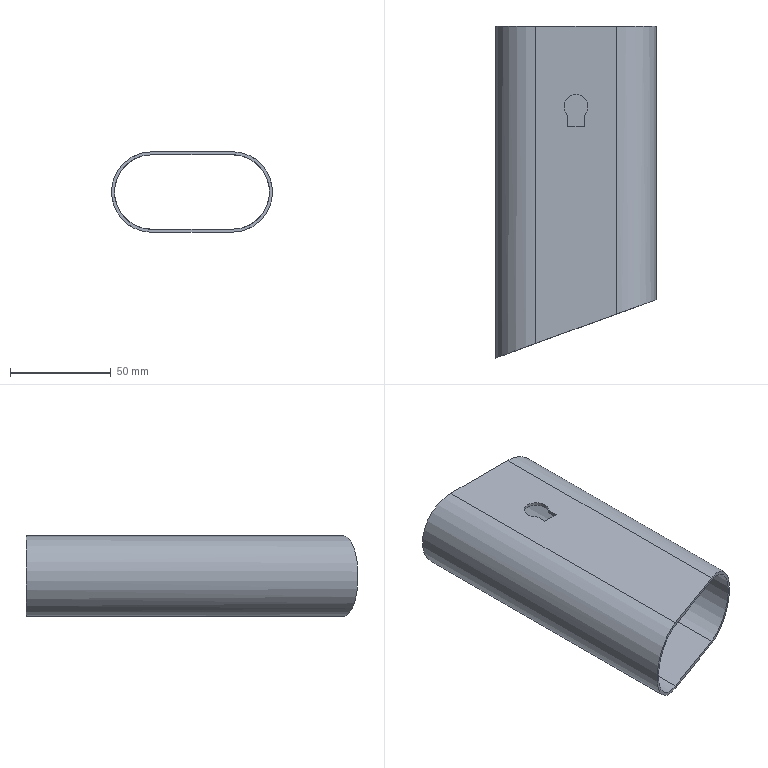Part | STEP file | 6100104R | 1 solid | 14 faces | box 80 x 165 x 40 mm | volume 45123 mm3 | plane 9 | cylinder 5 | commonest cylinder face diameters 37 x2 40 x2 12 x1
STEP:
#1=CARTESIAN_POINT('',(0.,0.,0.));
#2=DIRECTION('',(0.,0.,1.));
#3=DIRECTION('',(1.,0.,0.));
#4=AXIS2_PLACEMENT_3D('',#1,#2,#3);
#5=CARTESIAN_POINT('',(-20.,7.279,20.));
#6=VERTEX_POINT('',#5);
#7=CARTESIAN_POINT('',(-20.,7.279,-20.));
#8=VERTEX_POINT('',#7);
#9=CARTESIAN_POINT('',(-20.,7.279,20.));
#10=CARTESIAN_POINT('',(-60.,-7.279,20.));
#11=CARTESIAN_POINT('',(-60.,-7.279,-20.));
#12=CARTESIAN_POINT('',(-20.,7.279,-20.));
#13=(BOUNDED_CURVE()B_SPLINE_CURVE(3,(#9,#10,#11,#12),.UNSPECIFIED.,.F.,.F.)B_SPLINE_CURVE_WITH_KNOTS((4,4),(4.712,7.854),.PIECEWISE_BEZIER_KNOTS.)CURVE()GEOMETRIC_REPRESENTATION_ITEM()RATIONAL_B_SPLINE_CURVE((1.,0.3333,0.3333,1.))REPRESENTATION_ITEM(''));
#14=CARTESIAN_POINT('',(-20.,165.,0.));
#15=DIRECTION('',(0.,-1.,0.));
#16=DIRECTION('',(0.,0.,-1.));
#17=AXIS2_PLACEMENT_3D('',#14,#15,#16);
#18=CYLINDRICAL_SURFACE('',#17,20.);
#19=CARTESIAN_POINT('',(3.142,157.721));
#20=CARTESIAN_POINT('',(3.172,157.941));
#21=CARTESIAN_POINT('',(3.235,158.403));
#22=CARTESIAN_POINT('',(3.339,159.153));
#23=CARTESIAN_POINT('',(3.453,159.957));
#24=CARTESIAN_POINT('',(3.577,160.8));
#25=CARTESIAN_POINT('',(3.712,161.664));
#26=CARTESIAN_POINT('',(3.857,162.516));
#27=CARTESIAN_POINT('',(4.013,163.316));
#28=CARTESIAN_POINT('',(4.179,164.017));
#29=CARTESIAN_POINT('',(4.352,164.567));
#30=CARTESIAN_POINT('',(4.531,164.919));
#31=CARTESIAN_POINT('',(4.712,165.04));
#32=CARTESIAN_POINT('',(4.894,164.919));
#33=CARTESIAN_POINT('',(5.073,164.567));
#34=CARTESIAN_POINT('',(5.246,164.017));
#35=CARTESIAN_POINT('',(5.412,163.316));
#36=CARTESIAN_POINT('',(5.567,162.516));
#37=CARTESIAN_POINT('',(5.713,161.664));
#38=CARTESIAN_POINT('',(5.848,160.8));
#39=CARTESIAN_POINT('',(5.972,159.957));
#40=CARTESIAN_POINT('',(6.085,159.153));
#41=CARTESIAN_POINT('',(6.19,158.403));
#42=CARTESIAN_POINT('',(6.253,157.941));
#43=CARTESIAN_POINT('',(6.283,157.721));
#44=B_SPLINE_CURVE_WITH_KNOTS('',3,(#19,#20,#21,#22,#23,#24,#25,#26,#27,#28,#29,#30,#31,#32,#33,#34,#35,#36,#37,#38,#39,#40,#41,#42,#43),.UNSPECIFIED.,.F.,.F.,(4,1,1,1,1,1,1,1,1,1,1,1,1,1,1,1,1,1,1,1,1,1,4),(4.712,4.855,4.998,5.141,5.284,5.426,5.569,5.712,5.855,5.998,6.14,6.283,6.426,6.569,6.712,6.854,6.997,7.14,7.283,7.426,7.568,7.711,7.854),.QUASI_UNIFORM_KNOTS.);
#45=(GEOMETRIC_REPRESENTATION_CONTEXT(2)PARAMETRIC_REPRESENTATION_CONTEXT()REPRESENTATION_CONTEXT('',''));
#46=DEFINITIONAL_REPRESENTATION('',(#44),#45);
#47=PCURVE('',#18,#46);
#48=CARTESIAN_POINT('',(-40.,0.,-40.));
#49=DIRECTION('',(0.342,-0.9397,0.));
#50=DIRECTION('',(0.9397,0.342,0.));
#51=AXIS2_PLACEMENT_3D('',#48,#49,#50);
#52=PLANE('',#51);
#53=CARTESIAN_POINT('',(21.284,60.));
#54=CARTESIAN_POINT('',(-21.284,60.));
#55=CARTESIAN_POINT('',(-21.284,20.));
#56=CARTESIAN_POINT('',(21.284,20.));
#57=(BOUNDED_CURVE()B_SPLINE_CURVE(3,(#53,#54,#55,#56),.UNSPECIFIED.,.F.,.F.)B_SPLINE_CURVE_WITH_KNOTS((4,4),(4.712,7.854),.PIECEWISE_BEZIER_KNOTS.)CURVE()GEOMETRIC_REPRESENTATION_ITEM()RATIONAL_B_SPLINE_CURVE((1.,0.3333,0.3333,1.))REPRESENTATION_ITEM(''));
#58=(GEOMETRIC_REPRESENTATION_CONTEXT(2)PARAMETRIC_REPRESENTATION_CONTEXT()REPRESENTATION_CONTEXT('',''));
#59=DEFINITIONAL_REPRESENTATION('',(#57),#58);
#60=PCURVE('',#52,#59);
#61=SURFACE_CURVE('',#13,(#47,#60),.PCURVE_S1.);
#62=EDGE_CURVE('',#6,#8,#61,.T.);
#63=ORIENTED_EDGE('',*,*,#62,.F.);
#64=CARTESIAN_POINT('',(-20.,165.,20.));
#65=VERTEX_POINT('',#64);
#66=CARTESIAN_POINT('',(-20.,165.,20.));
#67=DIRECTION('',(0.,-1.,0.));
#68=VECTOR('',#67,1.);
#69=LINE('',#66,#68);
#70=CARTESIAN_POINT('',(3.142,0.));
#71=DIRECTION('',(0.,1.));
#72=VECTOR('',#71,1.);
#73=LINE('',#70,#72);
#74=(GEOMETRIC_REPRESENTATION_CONTEXT(2)PARAMETRIC_REPRESENTATION_CONTEXT()REPRESENTATION_CONTEXT('',''));
#75=DEFINITIONAL_REPRESENTATION('',(#73),#74);
#76=PCURVE('',#18,#75);
#77=CARTESIAN_POINT('',(-20.,165.,20.));
#78=DIRECTION('',(0.,0.,-1.));
#79=DIRECTION('',(-1.,0.,0.));
#80=AXIS2_PLACEMENT_3D('',#77,#78,#79);
#81=PLANE('',#80);
#82=CARTESIAN_POINT('',(0.,0.));
#83=DIRECTION('',(0.,-1.));
#84=VECTOR('',#83,1.);
#85=LINE('',#82,#84);
#86=(GEOMETRIC_REPRESENTATION_CONTEXT(2)PARAMETRIC_REPRESENTATION_CONTEXT()REPRESENTATION_CONTEXT('',''));
#87=DEFINITIONAL_REPRESENTATION('',(#85),#86);
#88=PCURVE('',#81,#87);
#89=SURFACE_CURVE('',#69,(#76,#88),.PCURVE_S1.);
#90=EDGE_CURVE('',#65,#6,#89,.T.);
#91=ORIENTED_EDGE('',*,*,#90,.F.);
#92=CARTESIAN_POINT('',(-20.,165.,-20.));
#93=VERTEX_POINT('',#92);
#94=CARTESIAN_POINT('',(-20.,165.,0.));
#95=DIRECTION('',(0.,1.,0.));
#96=DIRECTION('',(0.,0.,1.));
#97=AXIS2_PLACEMENT_3D('',#94,#95,#96);
#98=CIRCLE('',#97,20.);
#99=CARTESIAN_POINT('',(9.425,0.));
#100=DIRECTION('',(-1.,0.));
#101=VECTOR('',#100,1.);
#102=LINE('',#99,#101);
#103=(GEOMETRIC_REPRESENTATION_CONTEXT(2)PARAMETRIC_REPRESENTATION_CONTEXT()REPRESENTATION_CONTEXT('',''));
#104=DEFINITIONAL_REPRESENTATION('',(#102),#103);
#105=PCURVE('',#18,#104);
#106=CARTESIAN_POINT('',(-20.,165.,0.));
#107=DIRECTION('',(0.,1.,0.));
#108=DIRECTION('',(0.,0.,1.));
#109=AXIS2_PLACEMENT_3D('',#106,#107,#108);
#110=PLANE('',#109);
#111=CARTESIAN_POINT('',(0.,0.));
#112=DIRECTION('',(1.,0.));
#113=AXIS2_PLACEMENT_2D('',#111,#112);
#114=CIRCLE('',#113,20.);
#115=(GEOMETRIC_REPRESENTATION_CONTEXT(2)PARAMETRIC_REPRESENTATION_CONTEXT()REPRESENTATION_CONTEXT('',''));
#116=DEFINITIONAL_REPRESENTATION('',(#114),#115);
#117=PCURVE('',#110,#116);
#118=SURFACE_CURVE('',#98,(#105,#117),.PCURVE_S1.);
#119=EDGE_CURVE('',#93,#65,#118,.T.);
#120=ORIENTED_EDGE('',*,*,#119,.F.);
#121=CARTESIAN_POINT('',(-20.,165.,-20.));
#122=DIRECTION('',(0.,-1.,0.));
#123=VECTOR('',#122,1.);
#124=LINE('',#121,#123);
#125=CARTESIAN_POINT('',(6.283,0.));
#126=DIRECTION('',(0.,1.));
#127=VECTOR('',#126,1.);
#128=LINE('',#125,#127);
#129=(GEOMETRIC_REPRESENTATION_CONTEXT(2)PARAMETRIC_REPRESENTATION_CONTEXT()REPRESENTATION_CONTEXT('',''));
#130=DEFINITIONAL_REPRESENTATION('',(#128),#129);
#131=PCURVE('',#18,#130);
#132=CARTESIAN_POINT('',(-20.,165.,-20.));
#133=DIRECTION('',(0.,0.,1.));
#134=DIRECTION('',(1.,0.,0.));
#135=AXIS2_PLACEMENT_3D('',#132,#133,#134);
#136=PLANE('',#135);
#137=CARTESIAN_POINT('',(0.,0.));
#138=DIRECTION('',(0.,-1.));
#139=VECTOR('',#138,1.);
#140=LINE('',#137,#139);
#141=(GEOMETRIC_REPRESENTATION_CONTEXT(2)PARAMETRIC_REPRESENTATION_CONTEXT()REPRESENTATION_CONTEXT('',''));
#142=DEFINITIONAL_REPRESENTATION('',(#140),#141);
#143=PCURVE('',#136,#142);
#144=SURFACE_CURVE('',#124,(#131,#143),.PCURVE_S1.);
#145=EDGE_CURVE('',#93,#8,#144,.T.);
#146=ORIENTED_EDGE('',*,*,#145,.T.);
#147=EDGE_LOOP('',(#63,#91,#120,#146));
#148=FACE_BOUND('',#147,.T.);
#149=ADVANCED_FACE('',(#148),#18,.T.);
#150=CARTESIAN_POINT('',(4.,120.528,20.));
#151=VERTEX_POINT('',#150);
#152=CARTESIAN_POINT('',(-4.,120.528,20.));
#153=VERTEX_POINT('',#152);
#154=CARTESIAN_POINT('',(0.,125.,20.));
#155=DIRECTION('',(0.,0.,1.));
#156=DIRECTION('',(-1.,0.,0.));
#157=AXIS2_PLACEMENT_3D('',#154,#155,#156);
#158=CIRCLE('',#157,6.);
#159=CARTESIAN_POINT('',(-14.,-40.));
#160=CARTESIAN_POINT('',(-14.,-50.392));
#161=CARTESIAN_POINT('',(-23.,-45.196));
#162=CARTESIAN_POINT('',(-32.,-40.));
#163=CARTESIAN_POINT('',(-23.,-34.804));
#164=CARTESIAN_POINT('',(-14.,-29.608));
#165=CARTESIAN_POINT('',(-14.,-40.));
#166=(BOUNDED_CURVE()B_SPLINE_CURVE(2,(#159,#160,#161,#162,#163,#164,#165),.UNSPECIFIED.,.T.,.F.)B_SPLINE_CURVE_WITH_KNOTS((1,2,2,2,2,1),(-2.094,0.,2.094,4.189,6.283,8.378),.UNSPECIFIED.)CURVE()GEOMETRIC_REPRESENTATION_ITEM()RATIONAL_B_SPLINE_CURVE((1.,0.5,1.,0.5,1.,0.5,1.))REPRESENTATION_ITEM(''));
#167=(GEOMETRIC_REPRESENTATION_CONTEXT(2)PARAMETRIC_REPRESENTATION_CONTEXT()REPRESENTATION_CONTEXT('',''));
#168=DEFINITIONAL_REPRESENTATION('',(#166),#167);
#169=PCURVE('',#81,#168);
#170=CARTESIAN_POINT('',(0.,125.,40.));
#171=DIRECTION('',(0.,0.,-1.));
#172=DIRECTION('',(-1.,0.,0.));
#173=AXIS2_PLACEMENT_3D('',#170,#171,#172);
#174=CYLINDRICAL_SURFACE('',#173,6.);
#175=CARTESIAN_POINT('',(6.283,20.));
#176=DIRECTION('',(-1.,0.));
#177=VECTOR('',#176,1.);
#178=LINE('',#175,#177);
#179=(GEOMETRIC_REPRESENTATION_CONTEXT(2)PARAMETRIC_REPRESENTATION_CONTEXT()REPRESENTATION_CONTEXT('',''));
#180=DEFINITIONAL_REPRESENTATION('',(#178),#179);
#181=PCURVE('',#174,#180);
#182=SURFACE_CURVE('',#158,(#169,#181),.PCURVE_S1.);
#183=EDGE_CURVE('',#151,#153,#182,.T.);
#184=ORIENTED_EDGE('',*,*,#183,.F.);
#185=CARTESIAN_POINT('',(4.,115.,20.));
#186=VERTEX_POINT('',#185);
#187=CARTESIAN_POINT('',(4.,165.,20.));
#188=DIRECTION('',(0.,-1.,0.));
#189=VECTOR('',#188,1.);
#190=LINE('',#187,#189);
#191=CARTESIAN_POINT('',(-24.,0.));
#192=DIRECTION('',(0.,-1.));
#193=VECTOR('',#192,1.);
#194=LINE('',#191,#193);
#195=(GEOMETRIC_REPRESENTATION_CONTEXT(2)PARAMETRIC_REPRESENTATION_CONTEXT()REPRESENTATION_CONTEXT('',''));
#196=DEFINITIONAL_REPRESENTATION('',(#194),#195);
#197=PCURVE('',#81,#196);
#198=CARTESIAN_POINT('',(4.,120.528,40.));
#199=DIRECTION('',(1.,0.,0.));
#200=DIRECTION('',(0.,1.,0.));
#201=AXIS2_PLACEMENT_3D('',#198,#199,#200);
#202=PLANE('',#201);
#203=CARTESIAN_POINT('',(44.472,-20.));
#204=DIRECTION('',(-1.,0.));
#205=VECTOR('',#204,1.);
#206=LINE('',#203,#205);
#207=(GEOMETRIC_REPRESENTATION_CONTEXT(2)PARAMETRIC_REPRESENTATION_CONTEXT()REPRESENTATION_CONTEXT('',''));
#208=DEFINITIONAL_REPRESENTATION('',(#206),#207);
#209=PCURVE('',#202,#208);
#210=SURFACE_CURVE('',#190,(#197,#209),.PCURVE_S1.);
#211=EDGE_CURVE('',#151,#186,#210,.T.);
#212=ORIENTED_EDGE('',*,*,#211,.T.);
#213=CARTESIAN_POINT('',(-4.,115.,20.));
#214=VERTEX_POINT('',#213);
#215=CARTESIAN_POINT('',(-20.,115.,20.));
#216=DIRECTION('',(1.,0.,0.));
#217=VECTOR('',#216,1.);
#218=LINE('',#215,#217);
#219=CARTESIAN_POINT('',(0.,-50.));
#220=DIRECTION('',(-1.,0.));
#221=VECTOR('',#220,1.);
#222=LINE('',#219,#221);
#223=(GEOMETRIC_REPRESENTATION_CONTEXT(2)PARAMETRIC_REPRESENTATION_CONTEXT()REPRESENTATION_CONTEXT('',''));
#224=DEFINITIONAL_REPRESENTATION('',(#222),#223);
#225=PCURVE('',#81,#224);
#226=CARTESIAN_POINT('',(-4.,115.,40.));
#227=DIRECTION('',(0.,1.,0.));
#228=DIRECTION('',(0.,0.,1.));
#229=AXIS2_PLACEMENT_3D('',#226,#227,#228);
#230=PLANE('',#229);
#231=CARTESIAN_POINT('',(-20.,-16.));
#232=DIRECTION('',(0.,1.));
#233=VECTOR('',#232,1.);
#234=LINE('',#231,#233);
#235=(GEOMETRIC_REPRESENTATION_CONTEXT(2)PARAMETRIC_REPRESENTATION_CONTEXT()REPRESENTATION_CONTEXT('',''));
#236=DEFINITIONAL_REPRESENTATION('',(#234),#235);
#237=PCURVE('',#230,#236);
#238=SURFACE_CURVE('',#218,(#225,#237),.PCURVE_S1.);
#239=EDGE_CURVE('',#214,#186,#238,.T.);
#240=ORIENTED_EDGE('',*,*,#239,.F.);
#241=CARTESIAN_POINT('',(-4.,165.,20.));
#242=DIRECTION('',(0.,-1.,0.));
#243=VECTOR('',#242,1.);
#244=LINE('',#241,#243);
#245=CARTESIAN_POINT('',(-16.,0.));
#246=DIRECTION('',(0.,-1.));
#247=VECTOR('',#246,1.);
#248=LINE('',#245,#247);
#249=(GEOMETRIC_REPRESENTATION_CONTEXT(2)PARAMETRIC_REPRESENTATION_CONTEXT()REPRESENTATION_CONTEXT('',''));
#250=DEFINITIONAL_REPRESENTATION('',(#248),#249);
#251=PCURVE('',#81,#250);
#252=CARTESIAN_POINT('',(-4.,120.528,40.));
#253=DIRECTION('',(1.,0.,0.));
#254=DIRECTION('',(0.,1.,0.));
#255=AXIS2_PLACEMENT_3D('',#252,#253,#254);
#256=PLANE('',#255);
#257=CARTESIAN_POINT('',(44.472,-20.));
#258=DIRECTION('',(-1.,0.));
#259=VECTOR('',#258,1.);
#260=LINE('',#257,#259);
#261=(GEOMETRIC_REPRESENTATION_CONTEXT(2)PARAMETRIC_REPRESENTATION_CONTEXT()REPRESENTATION_CONTEXT('',''));
#262=DEFINITIONAL_REPRESENTATION('',(#260),#261);
#263=PCURVE('',#256,#262);
#264=SURFACE_CURVE('',#244,(#251,#263),.PCURVE_S1.);
#265=EDGE_CURVE('',#153,#214,#264,.T.);
#266=ORIENTED_EDGE('',*,*,#265,.F.);
#267=EDGE_LOOP('',(#184,#212,#240,#266));
#268=FACE_BOUND('',#267,.T.);
#269=CARTESIAN_POINT('',(20.,21.838,20.));
#270=VERTEX_POINT('',#269);
#271=CARTESIAN_POINT('',(30.69,25.729,20.));
#272=DIRECTION('',(-0.9397,-0.342,0.));
#273=VECTOR('',#272,1.);
#274=LINE('',#271,#273);
#275=CARTESIAN_POINT('',(-50.69,-139.271));
#276=DIRECTION('',(0.9397,-0.342));
#277=VECTOR('',#276,1.);
#278=LINE('',#275,#277);
#279=(GEOMETRIC_REPRESENTATION_CONTEXT(2)PARAMETRIC_REPRESENTATION_CONTEXT()REPRESENTATION_CONTEXT('',''));
#280=DEFINITIONAL_REPRESENTATION('',(#278),#279);
#281=PCURVE('',#81,#280);
#282=CARTESIAN_POINT('',(75.227,60.));
#283=DIRECTION('',(-1.,0.));
#284=VECTOR('',#283,1.);
#285=LINE('',#282,#284);
#286=(GEOMETRIC_REPRESENTATION_CONTEXT(2)PARAMETRIC_REPRESENTATION_CONTEXT()REPRESENTATION_CONTEXT('',''));
#287=DEFINITIONAL_REPRESENTATION('',(#285),#286);
#288=PCURVE('',#52,#287);
#289=SURFACE_CURVE('',#274,(#281,#288),.PCURVE_S1.);
#290=EDGE_CURVE('',#270,#6,#289,.T.);
#291=ORIENTED_EDGE('',*,*,#290,.F.);
#292=CARTESIAN_POINT('',(20.,165.,20.));
#293=VERTEX_POINT('',#292);
#294=CARTESIAN_POINT('',(20.,165.,20.));
#295=DIRECTION('',(0.,-1.,0.));
#296=VECTOR('',#295,1.);
#297=LINE('',#294,#296);
#298=CARTESIAN_POINT('',(-40.,0.));
#299=DIRECTION('',(0.,-1.));
#300=VECTOR('',#299,1.);
#301=LINE('',#298,#300);
#302=(GEOMETRIC_REPRESENTATION_CONTEXT(2)PARAMETRIC_REPRESENTATION_CONTEXT()REPRESENTATION_CONTEXT('',''));
#303=DEFINITIONAL_REPRESENTATION('',(#301),#302);
#304=PCURVE('',#81,#303);
#305=CARTESIAN_POINT('',(20.,165.,0.));
#306=DIRECTION('',(0.,-1.,0.));
#307=DIRECTION('',(0.,0.,-1.));
#308=AXIS2_PLACEMENT_3D('',#305,#306,#307);
#309=CYLINDRICAL_SURFACE('',#308,20.);
#310=CARTESIAN_POINT('',(3.142,0.));
#311=DIRECTION('',(0.,1.));
#312=VECTOR('',#311,1.);
#313=LINE('',#310,#312);
#314=(GEOMETRIC_REPRESENTATION_CONTEXT(2)PARAMETRIC_REPRESENTATION_CONTEXT()REPRESENTATION_CONTEXT('',''));
#315=DEFINITIONAL_REPRESENTATION('',(#313),#314);
#316=PCURVE('',#309,#315);
#317=SURFACE_CURVE('',#297,(#304,#316),.PCURVE_S1.);
#318=EDGE_CURVE('',#293,#270,#317,.T.);
#319=ORIENTED_EDGE('',*,*,#318,.F.);
#320=CARTESIAN_POINT('',(-20.,165.,20.));
#321=DIRECTION('',(1.,0.,0.));
#322=VECTOR('',#321,1.);
#323=LINE('',#320,#322);
#324=CARTESIAN_POINT('',(0.,0.));
#325=DIRECTION('',(-1.,0.));
#326=VECTOR('',#325,1.);
#327=LINE('',#324,#326);
#328=(GEOMETRIC_REPRESENTATION_CONTEXT(2)PARAMETRIC_REPRESENTATION_CONTEXT()REPRESENTATION_CONTEXT('',''));
#329=DEFINITIONAL_REPRESENTATION('',(#327),#328);
#330=PCURVE('',#81,#329);
#331=CARTESIAN_POINT('',(20.,0.));
#332=DIRECTION('',(0.,1.));
#333=VECTOR('',#332,1.);
#334=LINE('',#331,#333);
#335=(GEOMETRIC_REPRESENTATION_CONTEXT(2)PARAMETRIC_REPRESENTATION_CONTEXT()REPRESENTATION_CONTEXT('',''));
#336=DEFINITIONAL_REPRESENTATION('',(#334),#335);
#337=PCURVE('',#110,#336);
#338=SURFACE_CURVE('',#323,(#330,#337),.PCURVE_S1.);
#339=EDGE_CURVE('',#65,#293,#338,.T.);
#340=ORIENTED_EDGE('',*,*,#339,.F.);
#341=ORIENTED_EDGE('',*,*,#90,.T.);
#342=EDGE_LOOP('',(#291,#319,#340,#341));
#343=FACE_BOUND('',#342,.T.);
#344=ADVANCED_FACE('',(#268,#343),#81,.F.);
#345=ORIENTED_EDGE('',*,*,#318,.T.);
#346=CARTESIAN_POINT('',(20.,21.838,-20.));
#347=VERTEX_POINT('',#346);
#348=CARTESIAN_POINT('',(20.,21.838,-20.));
#349=CARTESIAN_POINT('',(60.,36.397,-20.));
#350=CARTESIAN_POINT('',(60.,36.397,20.));
#351=CARTESIAN_POINT('',(20.,21.838,20.));
#352=(BOUNDED_CURVE()B_SPLINE_CURVE(3,(#348,#349,#350,#351),.UNSPECIFIED.,.F.,.F.)B_SPLINE_CURVE_WITH_KNOTS((4,4),(1.571,4.712),.PIECEWISE_BEZIER_KNOTS.)CURVE()GEOMETRIC_REPRESENTATION_ITEM()RATIONAL_B_SPLINE_CURVE((1.,0.3333,0.3333,1.))REPRESENTATION_ITEM(''));
#353=CARTESIAN_POINT('',(0.,143.162));
#354=CARTESIAN_POINT('',(0.0303,142.942));
#355=CARTESIAN_POINT('',(0.09367,142.48));
#356=CARTESIAN_POINT('',(0.1977,141.729));
#357=CARTESIAN_POINT('',(0.3115,140.926));
#358=CARTESIAN_POINT('',(0.4356,140.082));
#359=CARTESIAN_POINT('',(0.5703,139.219));
#360=CARTESIAN_POINT('',(0.7158,138.367));
#361=CARTESIAN_POINT('',(0.8717,137.566));
#362=CARTESIAN_POINT('',(1.037,136.865));
#363=CARTESIAN_POINT('',(1.21,136.315));
#364=CARTESIAN_POINT('',(1.389,135.963));
#365=CARTESIAN_POINT('',(1.571,135.842));
#366=CARTESIAN_POINT('',(1.753,135.963));
#367=CARTESIAN_POINT('',(1.931,136.315));
#368=CARTESIAN_POINT('',(2.105,136.865));
#369=CARTESIAN_POINT('',(2.27,137.566));
#370=CARTESIAN_POINT('',(2.426,138.367));
#371=CARTESIAN_POINT('',(2.571,139.219));
#372=CARTESIAN_POINT('',(2.706,140.082));
#373=CARTESIAN_POINT('',(2.83,140.926));
#374=CARTESIAN_POINT('',(2.944,141.729));
#375=CARTESIAN_POINT('',(3.048,142.48));
#376=CARTESIAN_POINT('',(3.111,142.942));
#377=CARTESIAN_POINT('',(3.142,143.162));
#378=B_SPLINE_CURVE_WITH_KNOTS('',3,(#353,#354,#355,#356,#357,#358,#359,#360,#361,#362,#363,#364,#365,#366,#367,#368,#369,#370,#371,#372,#373,#374,#375,#376,#377),.UNSPECIFIED.,.F.,.F.,(4,1,1,1,1,1,1,1,1,1,1,1,1,1,1,1,1,1,1,1,1,1,4),(1.571,1.714,1.856,1.999,2.142,2.285,2.428,2.57,2.713,2.856,2.999,3.142,3.284,3.427,3.57,3.713,3.856,3.998,4.141,4.284,4.427,4.57,4.712),.QUASI_UNIFORM_KNOTS.);
#379=(GEOMETRIC_REPRESENTATION_CONTEXT(2)PARAMETRIC_REPRESENTATION_CONTEXT()REPRESENTATION_CONTEXT('',''));
#380=DEFINITIONAL_REPRESENTATION('',(#378),#379);
#381=PCURVE('',#309,#380);
#382=CARTESIAN_POINT('',(63.851,20.));
#383=CARTESIAN_POINT('',(106.418,20.));
#384=CARTESIAN_POINT('',(106.418,60.));
#385=CARTESIAN_POINT('',(63.851,60.));
#386=(BOUNDED_CURVE()B_SPLINE_CURVE(3,(#382,#383,#384,#385),.UNSPECIFIED.,.F.,.F.)B_SPLINE_CURVE_WITH_KNOTS((4,4),(1.571,4.712),.PIECEWISE_BEZIER_KNOTS.)CURVE()GEOMETRIC_REPRESENTATION_ITEM()RATIONAL_B_SPLINE_CURVE((1.,0.3333,0.3333,1.))REPRESENTATION_ITEM(''));
#387=(GEOMETRIC_REPRESENTATION_CONTEXT(2)PARAMETRIC_REPRESENTATION_CONTEXT()REPRESENTATION_CONTEXT('',''));
#388=DEFINITIONAL_REPRESENTATION('',(#386),#387);
#389=PCURVE('',#52,#388);
#390=SURFACE_CURVE('',#352,(#381,#389),.PCURVE_S1.);
#391=EDGE_CURVE('',#347,#270,#390,.T.);
#392=ORIENTED_EDGE('',*,*,#391,.F.);
#393=CARTESIAN_POINT('',(20.,165.,-20.));
#394=VERTEX_POINT('',#393);
#395=CARTESIAN_POINT('',(20.,165.,-20.));
#396=DIRECTION('',(0.,-1.,0.));
#397=VECTOR('',#396,1.);
#398=LINE('',#395,#397);
#399=CARTESIAN_POINT('',(0.,0.));
#400=DIRECTION('',(0.,1.));
#401=VECTOR('',#400,1.);
#402=LINE('',#399,#401);
#403=(GEOMETRIC_REPRESENTATION_CONTEXT(2)PARAMETRIC_REPRESENTATION_CONTEXT()REPRESENTATION_CONTEXT('',''));
#404=DEFINITIONAL_REPRESENTATION('',(#402),#403);
#405=PCURVE('',#309,#404);
#406=CARTESIAN_POINT('',(40.,0.));
#407=DIRECTION('',(0.,-1.));
#408=VECTOR('',#407,1.);
#409=LINE('',#406,#408);
#410=(GEOMETRIC_REPRESENTATION_CONTEXT(2)PARAMETRIC_REPRESENTATION_CONTEXT()REPRESENTATION_CONTEXT('',''));
#411=DEFINITIONAL_REPRESENTATION('',(#409),#410);
#412=PCURVE('',#136,#411);
#413=SURFACE_CURVE('',#398,(#405,#412),.PCURVE_S1.);
#414=EDGE_CURVE('',#394,#347,#413,.T.);
#415=ORIENTED_EDGE('',*,*,#414,.F.);
#416=CARTESIAN_POINT('',(20.,165.,0.));
#417=DIRECTION('',(0.,1.,0.));
#418=DIRECTION('',(0.,0.,1.));
#419=AXIS2_PLACEMENT_3D('',#416,#417,#418);
#420=CIRCLE('',#419,20.);
#421=CARTESIAN_POINT('',(3.142,0.));
#422=DIRECTION('',(-1.,0.));
#423=VECTOR('',#422,1.);
#424=LINE('',#421,#423);
#425=(GEOMETRIC_REPRESENTATION_CONTEXT(2)PARAMETRIC_REPRESENTATION_CONTEXT()REPRESENTATION_CONTEXT('',''));
#426=DEFINITIONAL_REPRESENTATION('',(#424),#425);
#427=PCURVE('',#309,#426);
#428=CARTESIAN_POINT('',(0.,40.));
#429=DIRECTION('',(1.,0.));
#430=AXIS2_PLACEMENT_2D('',#428,#429);
#431=CIRCLE('',#430,20.);
#432=(GEOMETRIC_REPRESENTATION_CONTEXT(2)PARAMETRIC_REPRESENTATION_CONTEXT()REPRESENTATION_CONTEXT('',''));
#433=DEFINITIONAL_REPRESENTATION('',(#431),#432);
#434=PCURVE('',#110,#433);
#435=SURFACE_CURVE('',#420,(#427,#434),.PCURVE_S1.);
#436=EDGE_CURVE('',#293,#394,#435,.T.);
#437=ORIENTED_EDGE('',*,*,#436,.F.);
#438=EDGE_LOOP('',(#345,#392,#415,#437));
#439=FACE_BOUND('',#438,.T.);
#440=ADVANCED_FACE('',(#439),#309,.T.);
#441=CARTESIAN_POINT('',(30.69,25.729,-20.));
#442=DIRECTION('',(0.9397,0.342,0.));
#443=VECTOR('',#442,1.);
#444=LINE('',#441,#443);
#445=CARTESIAN_POINT('',(50.69,-139.271));
#446=DIRECTION('',(0.9397,0.342));
#447=VECTOR('',#446,1.);
#448=LINE('',#445,#447);
#449=(GEOMETRIC_REPRESENTATION_CONTEXT(2)PARAMETRIC_REPRESENTATION_CONTEXT()REPRESENTATION_CONTEXT('',''));
#450=DEFINITIONAL_REPRESENTATION('',(#448),#449);
#451=PCURVE('',#136,#450);
#452=CARTESIAN_POINT('',(75.227,20.));
#453=DIRECTION('',(1.,0.));
#454=VECTOR('',#453,1.);
#455=LINE('',#452,#454);
#456=(GEOMETRIC_REPRESENTATION_CONTEXT(2)PARAMETRIC_REPRESENTATION_CONTEXT()REPRESENTATION_CONTEXT('',''));
#457=DEFINITIONAL_REPRESENTATION('',(#455),#456);
#458=PCURVE('',#52,#457);
#459=SURFACE_CURVE('',#444,(#451,#458),.PCURVE_S1.);
#460=EDGE_CURVE('',#8,#347,#459,.T.);
#461=ORIENTED_EDGE('',*,*,#460,.F.);
#462=ORIENTED_EDGE('',*,*,#145,.F.);
#463=CARTESIAN_POINT('',(-20.,165.,-20.));
#464=DIRECTION('',(-1.,0.,0.));
#465=VECTOR('',#464,1.);
#466=LINE('',#463,#465);
#467=CARTESIAN_POINT('',(0.,0.));
#468=DIRECTION('',(-1.,0.));
#469=VECTOR('',#468,1.);
#470=LINE('',#467,#469);
#471=(GEOMETRIC_REPRESENTATION_CONTEXT(2)PARAMETRIC_REPRESENTATION_CONTEXT()REPRESENTATION_CONTEXT('',''));
#472=DEFINITIONAL_REPRESENTATION('',(#470),#471);
#473=PCURVE('',#136,#472);
#474=CARTESIAN_POINT('',(-20.,0.));
#475=DIRECTION('',(0.,-1.));
#476=VECTOR('',#475,1.);
#477=LINE('',#474,#476);
#478=(GEOMETRIC_REPRESENTATION_CONTEXT(2)PARAMETRIC_REPRESENTATION_CONTEXT()REPRESENTATION_CONTEXT('',''));
#479=DEFINITIONAL_REPRESENTATION('',(#477),#478);
#480=PCURVE('',#110,#479);
#481=SURFACE_CURVE('',#466,(#473,#480),.PCURVE_S1.);
#482=EDGE_CURVE('',#394,#93,#481,.T.);
#483=ORIENTED_EDGE('',*,*,#482,.F.);
#484=ORIENTED_EDGE('',*,*,#414,.T.);
#485=EDGE_LOOP('',(#461,#462,#483,#484));
#486=FACE_BOUND('',#485,.T.);
#487=ADVANCED_FACE('',(#486),#136,.F.);
#488=CARTESIAN_POINT('',(-20.,165.,-18.5));
#489=VERTEX_POINT('',#488);
#490=CARTESIAN_POINT('',(-20.,165.,18.5));
#491=VERTEX_POINT('',#490);
#492=CARTESIAN_POINT('',(-20.,165.,0.));
#493=DIRECTION('',(0.,1.,0.));
#494=DIRECTION('',(0.,0.,1.));
#495=AXIS2_PLACEMENT_3D('',#492,#493,#494);
#496=CIRCLE('',#495,18.5);
#497=CARTESIAN_POINT('',(-20.,165.,0.));
#498=DIRECTION('',(0.,-1.,0.));
#499=DIRECTION('',(0.,0.,-1.));
#500=AXIS2_PLACEMENT_3D('',#497,#498,#499);
#501=CYLINDRICAL_SURFACE('',#500,18.5);
#502=CARTESIAN_POINT('',(9.425,0.));
#503=DIRECTION('',(-1.,0.));
#504=VECTOR('',#503,1.);
#505=LINE('',#502,#504);
#506=(GEOMETRIC_REPRESENTATION_CONTEXT(2)PARAMETRIC_REPRESENTATION_CONTEXT()REPRESENTATION_CONTEXT('',''));
#507=DEFINITIONAL_REPRESENTATION('',(#505),#506);
#508=PCURVE('',#501,#507);
#509=CARTESIAN_POINT('',(0.,0.));
#510=DIRECTION('',(1.,0.));
#511=AXIS2_PLACEMENT_2D('',#509,#510);
#512=CIRCLE('',#511,18.5);
#513=(GEOMETRIC_REPRESENTATION_CONTEXT(2)PARAMETRIC_REPRESENTATION_CONTEXT()REPRESENTATION_CONTEXT('',''));
#514=DEFINITIONAL_REPRESENTATION('',(#512),#513);
#515=PCURVE('',#110,#514);
#516=SURFACE_CURVE('',#496,(#508,#515),.PCURVE_S1.);
#517=EDGE_CURVE('',#489,#491,#516,.T.);
#518=ORIENTED_EDGE('',*,*,#517,.F.);
#519=CARTESIAN_POINT('',(-20.,7.279,-18.5));
#520=VERTEX_POINT('',#519);
#521=CARTESIAN_POINT('',(-20.,165.,-18.5));
#522=DIRECTION('',(0.,-1.,0.));
#523=VECTOR('',#522,1.);
#524=LINE('',#521,#523);
#525=CARTESIAN_POINT('',(6.283,0.));
#526=DIRECTION('',(0.,1.));
#527=VECTOR('',#526,1.);
#528=LINE('',#525,#527);
#529=(GEOMETRIC_REPRESENTATION_CONTEXT(2)PARAMETRIC_REPRESENTATION_CONTEXT()REPRESENTATION_CONTEXT('',''));
#530=DEFINITIONAL_REPRESENTATION('',(#528),#529);
#531=PCURVE('',#501,#530);
#532=CARTESIAN_POINT('',(-20.,165.,-18.5));
#533=DIRECTION('',(0.,0.,1.));
#534=DIRECTION('',(1.,0.,0.));
#535=AXIS2_PLACEMENT_3D('',#532,#533,#534);
#536=PLANE('',#535);
#537=CARTESIAN_POINT('',(0.,0.));
#538=DIRECTION('',(0.,-1.));
#539=VECTOR('',#538,1.);
#540=LINE('',#537,#539);
#541=(GEOMETRIC_REPRESENTATION_CONTEXT(2)PARAMETRIC_REPRESENTATION_CONTEXT()REPRESENTATION_CONTEXT('',''));
#542=DEFINITIONAL_REPRESENTATION('',(#540),#541);
#543=PCURVE('',#536,#542);
#544=SURFACE_CURVE('',#524,(#531,#543),.PCURVE_S1.);
#545=EDGE_CURVE('',#489,#520,#544,.T.);
#546=ORIENTED_EDGE('',*,*,#545,.T.);
#547=CARTESIAN_POINT('',(-20.,7.279,18.5));
#548=VERTEX_POINT('',#547);
#549=CARTESIAN_POINT('',(-20.,7.279,18.5));
#550=CARTESIAN_POINT('',(-57.,-6.187,18.5));
#551=CARTESIAN_POINT('',(-57.,-6.187,-18.5));
#552=CARTESIAN_POINT('',(-20.,7.279,-18.5));
#553=(BOUNDED_CURVE()B_SPLINE_CURVE(3,(#549,#550,#551,#552),.UNSPECIFIED.,.F.,.F.)B_SPLINE_CURVE_WITH_KNOTS((4,4),(4.712,7.854),.PIECEWISE_BEZIER_KNOTS.)CURVE()GEOMETRIC_REPRESENTATION_ITEM()RATIONAL_B_SPLINE_CURVE((1.,0.3333,0.3333,1.))REPRESENTATION_ITEM(''));
#554=CARTESIAN_POINT('',(3.142,157.721));
#555=CARTESIAN_POINT('',(3.172,157.924));
#556=CARTESIAN_POINT('',(3.235,158.352));
#557=CARTESIAN_POINT('',(3.339,159.046));
#558=CARTESIAN_POINT('',(3.453,159.789));
#559=CARTESIAN_POINT('',(3.577,160.569));
#560=CARTESIAN_POINT('',(3.712,161.368));
#561=CARTESIAN_POINT('',(3.857,162.156));
#562=CARTESIAN_POINT('',(4.013,162.897));
#563=CARTESIAN_POINT('',(4.179,163.545));
#564=CARTESIAN_POINT('',(4.352,164.054));
#565=CARTESIAN_POINT('',(4.531,164.379));
#566=CARTESIAN_POINT('',(4.712,164.491));
#567=CARTESIAN_POINT('',(4.894,164.379));
#568=CARTESIAN_POINT('',(5.073,164.054));
#569=CARTESIAN_POINT('',(5.246,163.545));
#570=CARTESIAN_POINT('',(5.412,162.897));
#571=CARTESIAN_POINT('',(5.567,162.156));
#572=CARTESIAN_POINT('',(5.713,161.368));
#573=CARTESIAN_POINT('',(5.848,160.569));
#574=CARTESIAN_POINT('',(5.972,159.789));
#575=CARTESIAN_POINT('',(6.085,159.046));
#576=CARTESIAN_POINT('',(6.19,158.352));
#577=CARTESIAN_POINT('',(6.253,157.924));
#578=CARTESIAN_POINT('',(6.283,157.721));
#579=B_SPLINE_CURVE_WITH_KNOTS('',3,(#554,#555,#556,#557,#558,#559,#560,#561,#562,#563,#564,#565,#566,#567,#568,#569,#570,#571,#572,#573,#574,#575,#576,#577,#578),.UNSPECIFIED.,.F.,.F.,(4,1,1,1,1,1,1,1,1,1,1,1,1,1,1,1,1,1,1,1,1,1,4),(4.712,4.855,4.998,5.141,5.284,5.426,5.569,5.712,5.855,5.998,6.14,6.283,6.426,6.569,6.712,6.854,6.997,7.14,7.283,7.426,7.568,7.711,7.854),.QUASI_UNIFORM_KNOTS.);
#580=(GEOMETRIC_REPRESENTATION_CONTEXT(2)PARAMETRIC_REPRESENTATION_CONTEXT()REPRESENTATION_CONTEXT('',''));
#581=DEFINITIONAL_REPRESENTATION('',(#579),#580);
#582=PCURVE('',#501,#581);
#583=CARTESIAN_POINT('',(21.284,58.5));
#584=CARTESIAN_POINT('',(-18.091,58.5));
#585=CARTESIAN_POINT('',(-18.091,21.5));
#586=CARTESIAN_POINT('',(21.284,21.5));
#587=(BOUNDED_CURVE()B_SPLINE_CURVE(3,(#583,#584,#585,#586),.UNSPECIFIED.,.F.,.F.)B_SPLINE_CURVE_WITH_KNOTS((4,4),(4.712,7.854),.PIECEWISE_BEZIER_KNOTS.)CURVE()GEOMETRIC_REPRESENTATION_ITEM()RATIONAL_B_SPLINE_CURVE((1.,0.3333,0.3333,1.))REPRESENTATION_ITEM(''));
#588=(GEOMETRIC_REPRESENTATION_CONTEXT(2)PARAMETRIC_REPRESENTATION_CONTEXT()REPRESENTATION_CONTEXT('',''));
#589=DEFINITIONAL_REPRESENTATION('',(#587),#588);
#590=PCURVE('',#52,#589);
#591=SURFACE_CURVE('',#553,(#582,#590),.PCURVE_S1.);
#592=EDGE_CURVE('',#548,#520,#591,.T.);
#593=ORIENTED_EDGE('',*,*,#592,.F.);
#594=CARTESIAN_POINT('',(-20.,165.,18.5));
#595=DIRECTION('',(0.,-1.,0.));
#596=VECTOR('',#595,1.);
#597=LINE('',#594,#596);
#598=CARTESIAN_POINT('',(3.142,0.));
#599=DIRECTION('',(0.,1.));
#600=VECTOR('',#599,1.);
#601=LINE('',#598,#600);
#602=(GEOMETRIC_REPRESENTATION_CONTEXT(2)PARAMETRIC_REPRESENTATION_CONTEXT()REPRESENTATION_CONTEXT('',''));
#603=DEFINITIONAL_REPRESENTATION('',(#601),#602);
#604=PCURVE('',#501,#603);
#605=CARTESIAN_POINT('',(-20.,165.,18.5));
#606=DIRECTION('',(0.,0.,-1.));
#607=DIRECTION('',(-1.,0.,0.));
#608=AXIS2_PLACEMENT_3D('',#605,#606,#607);
#609=PLANE('',#608);
#610=CARTESIAN_POINT('',(0.,0.));
#611=DIRECTION('',(0.,-1.));
#612=VECTOR('',#611,1.);
#613=LINE('',#610,#612);
#614=(GEOMETRIC_REPRESENTATION_CONTEXT(2)PARAMETRIC_REPRESENTATION_CONTEXT()REPRESENTATION_CONTEXT('',''));
#615=DEFINITIONAL_REPRESENTATION('',(#613),#614);
#616=PCURVE('',#609,#615);
#617=SURFACE_CURVE('',#597,(#604,#616),.PCURVE_S1.);
#618=EDGE_CURVE('',#491,#548,#617,.T.);
#619=ORIENTED_EDGE('',*,*,#618,.F.);
#620=EDGE_LOOP('',(#518,#546,#593,#619));
#621=FACE_BOUND('',#620,.F.);
#622=ADVANCED_FACE('',(#621),#501,.F.);
#623=CARTESIAN_POINT('',(4.,120.528,18.5));
#624=VERTEX_POINT('',#623);
#625=CARTESIAN_POINT('',(4.,115.,18.5));
#626=VERTEX_POINT('',#625);
#627=CARTESIAN_POINT('',(4.,165.,18.5));
#628=DIRECTION('',(0.,-1.,0.));
#629=VECTOR('',#628,1.);
#630=LINE('',#627,#629);
#631=CARTESIAN_POINT('',(-24.,0.));
#632=DIRECTION('',(0.,-1.));
#633=VECTOR('',#632,1.);
#634=LINE('',#631,#633);
#635=(GEOMETRIC_REPRESENTATION_CONTEXT(2)PARAMETRIC_REPRESENTATION_CONTEXT()REPRESENTATION_CONTEXT('',''));
#636=DEFINITIONAL_REPRESENTATION('',(#634),#635);
#637=PCURVE('',#609,#636);
#638=CARTESIAN_POINT('',(44.472,-21.5));
#639=DIRECTION('',(-1.,0.));
#640=VECTOR('',#639,1.);
#641=LINE('',#638,#640);
#642=(GEOMETRIC_REPRESENTATION_CONTEXT(2)PARAMETRIC_REPRESENTATION_CONTEXT()REPRESENTATION_CONTEXT('',''));
#643=DEFINITIONAL_REPRESENTATION('',(#641),#642);
#644=PCURVE('',#202,#643);
#645=SURFACE_CURVE('',#630,(#637,#644),.PCURVE_S1.);
#646=EDGE_CURVE('',#624,#626,#645,.T.);
#647=ORIENTED_EDGE('',*,*,#646,.F.);
#648=CARTESIAN_POINT('',(-4.,120.528,18.5));
#649=VERTEX_POINT('',#648);
#650=CARTESIAN_POINT('',(0.,125.,18.5));
#651=DIRECTION('',(0.,0.,1.));
#652=DIRECTION('',(-1.,0.,0.));
#653=AXIS2_PLACEMENT_3D('',#650,#651,#652);
#654=CIRCLE('',#653,6.);
#655=CARTESIAN_POINT('',(-14.,-40.));
#656=CARTESIAN_POINT('',(-14.,-50.392));
#657=CARTESIAN_POINT('',(-23.,-45.196));
#658=CARTESIAN_POINT('',(-32.,-40.));
#659=CARTESIAN_POINT('',(-23.,-34.804));
#660=CARTESIAN_POINT('',(-14.,-29.608));
#661=CARTESIAN_POINT('',(-14.,-40.));
#662=(BOUNDED_CURVE()B_SPLINE_CURVE(2,(#655,#656,#657,#658,#659,#660,#661),.UNSPECIFIED.,.T.,.F.)B_SPLINE_CURVE_WITH_KNOTS((1,2,2,2,2,1),(-2.094,0.,2.094,4.189,6.283,8.378),.UNSPECIFIED.)CURVE()GEOMETRIC_REPRESENTATION_ITEM()RATIONAL_B_SPLINE_CURVE((1.,0.5,1.,0.5,1.,0.5,1.))REPRESENTATION_ITEM(''));
#663=(GEOMETRIC_REPRESENTATION_CONTEXT(2)PARAMETRIC_REPRESENTATION_CONTEXT()REPRESENTATION_CONTEXT('',''));
#664=DEFINITIONAL_REPRESENTATION('',(#662),#663);
#665=PCURVE('',#609,#664);
#666=CARTESIAN_POINT('',(6.283,21.5));
#667=DIRECTION('',(-1.,0.));
#668=VECTOR('',#667,1.);
#669=LINE('',#666,#668);
#670=(GEOMETRIC_REPRESENTATION_CONTEXT(2)PARAMETRIC_REPRESENTATION_CONTEXT()REPRESENTATION_CONTEXT('',''));
#671=DEFINITIONAL_REPRESENTATION('',(#669),#670);
#672=PCURVE('',#174,#671);
#673=SURFACE_CURVE('',#654,(#665,#672),.PCURVE_S1.);
#674=EDGE_CURVE('',#624,#649,#673,.T.);
#675=ORIENTED_EDGE('',*,*,#674,.T.);
#676=CARTESIAN_POINT('',(-4.,115.,18.5));
#677=VERTEX_POINT('',#676);
#678=CARTESIAN_POINT('',(-4.,165.,18.5));
#679=DIRECTION('',(0.,-1.,0.));
#680=VECTOR('',#679,1.);
#681=LINE('',#678,#680);
#682=CARTESIAN_POINT('',(-16.,0.));
#683=DIRECTION('',(0.,-1.));
#684=VECTOR('',#683,1.);
#685=LINE('',#682,#684);
#686=(GEOMETRIC_REPRESENTATION_CONTEXT(2)PARAMETRIC_REPRESENTATION_CONTEXT()REPRESENTATION_CONTEXT('',''));
#687=DEFINITIONAL_REPRESENTATION('',(#685),#686);
#688=PCURVE('',#609,#687);
#689=CARTESIAN_POINT('',(44.472,-21.5));
#690=DIRECTION('',(-1.,0.));
#691=VECTOR('',#690,1.);
#692=LINE('',#689,#691);
#693=(GEOMETRIC_REPRESENTATION_CONTEXT(2)PARAMETRIC_REPRESENTATION_CONTEXT()REPRESENTATION_CONTEXT('',''));
#694=DEFINITIONAL_REPRESENTATION('',(#692),#693);
#695=PCURVE('',#256,#694);
#696=SURFACE_CURVE('',#681,(#688,#695),.PCURVE_S1.);
#697=EDGE_CURVE('',#649,#677,#696,.T.);
#698=ORIENTED_EDGE('',*,*,#697,.T.);
#699=CARTESIAN_POINT('',(-20.,115.,18.5));
#700=DIRECTION('',(1.,0.,0.));
#701=VECTOR('',#700,1.);
#702=LINE('',#699,#701);
#703=CARTESIAN_POINT('',(0.,-50.));
#704=DIRECTION('',(-1.,0.));
#705=VECTOR('',#704,1.);
#706=LINE('',#703,#705);
#707=(GEOMETRIC_REPRESENTATION_CONTEXT(2)PARAMETRIC_REPRESENTATION_CONTEXT()REPRESENTATION_CONTEXT('',''));
#708=DEFINITIONAL_REPRESENTATION('',(#706),#707);
#709=PCURVE('',#609,#708);
#710=CARTESIAN_POINT('',(-21.5,-16.));
#711=DIRECTION('',(0.,1.));
#712=VECTOR('',#711,1.);
#713=LINE('',#710,#712);
#714=(GEOMETRIC_REPRESENTATION_CONTEXT(2)PARAMETRIC_REPRESENTATION_CONTEXT()REPRESENTATION_CONTEXT('',''));
#715=DEFINITIONAL_REPRESENTATION('',(#713),#714);
#716=PCURVE('',#230,#715);
#717=SURFACE_CURVE('',#702,(#709,#716),.PCURVE_S1.);
#718=EDGE_CURVE('',#677,#626,#717,.T.);
#719=ORIENTED_EDGE('',*,*,#718,.T.);
#720=EDGE_LOOP('',(#647,#675,#698,#719));
#721=FACE_BOUND('',#720,.T.);
#722=CARTESIAN_POINT('',(20.,165.,18.5));
#723=VERTEX_POINT('',#722);
#724=CARTESIAN_POINT('',(20.,21.838,18.5));
#725=VERTEX_POINT('',#724);
#726=CARTESIAN_POINT('',(20.,165.,18.5));
#727=DIRECTION('',(0.,-1.,0.));
#728=VECTOR('',#727,1.);
#729=LINE('',#726,#728);
#730=CARTESIAN_POINT('',(-40.,0.));
#731=DIRECTION('',(0.,-1.));
#732=VECTOR('',#731,1.);
#733=LINE('',#730,#732);
#734=(GEOMETRIC_REPRESENTATION_CONTEXT(2)PARAMETRIC_REPRESENTATION_CONTEXT()REPRESENTATION_CONTEXT('',''));
#735=DEFINITIONAL_REPRESENTATION('',(#733),#734);
#736=PCURVE('',#609,#735);
#737=CARTESIAN_POINT('',(20.,165.,0.));
#738=DIRECTION('',(0.,-1.,0.));
#739=DIRECTION('',(0.,0.,-1.));
#740=AXIS2_PLACEMENT_3D('',#737,#738,#739);
#741=CYLINDRICAL_SURFACE('',#740,18.5);
#742=CARTESIAN_POINT('',(3.142,0.));
#743=DIRECTION('',(0.,1.));
#744=VECTOR('',#743,1.);
#745=LINE('',#742,#744);
#746=(GEOMETRIC_REPRESENTATION_CONTEXT(2)PARAMETRIC_REPRESENTATION_CONTEXT()REPRESENTATION_CONTEXT('',''));
#747=DEFINITIONAL_REPRESENTATION('',(#745),#746);
#748=PCURVE('',#741,#747);
#749=SURFACE_CURVE('',#729,(#736,#748),.PCURVE_S1.);
#750=EDGE_CURVE('',#723,#725,#749,.T.);
#751=ORIENTED_EDGE('',*,*,#750,.T.);
#752=CARTESIAN_POINT('',(30.69,25.729,18.5));
#753=DIRECTION('',(-0.9397,-0.342,0.));
#754=VECTOR('',#753,1.);
#755=LINE('',#752,#754);
#756=CARTESIAN_POINT('',(-50.69,-139.271));
#757=DIRECTION('',(0.9397,-0.342));
#758=VECTOR('',#757,1.);
#759=LINE('',#756,#758);
#760=(GEOMETRIC_REPRESENTATION_CONTEXT(2)PARAMETRIC_REPRESENTATION_CONTEXT()REPRESENTATION_CONTEXT('',''));
#761=DEFINITIONAL_REPRESENTATION('',(#759),#760);
#762=PCURVE('',#609,#761);
#763=CARTESIAN_POINT('',(75.227,58.5));
#764=DIRECTION('',(-1.,0.));
#765=VECTOR('',#764,1.);
#766=LINE('',#763,#765);
#767=(GEOMETRIC_REPRESENTATION_CONTEXT(2)PARAMETRIC_REPRESENTATION_CONTEXT()REPRESENTATION_CONTEXT('',''));
#768=DEFINITIONAL_REPRESENTATION('',(#766),#767);
#769=PCURVE('',#52,#768);
#770=SURFACE_CURVE('',#755,(#762,#769),.PCURVE_S1.);
#771=EDGE_CURVE('',#725,#548,#770,.T.);
#772=ORIENTED_EDGE('',*,*,#771,.T.);
#773=ORIENTED_EDGE('',*,*,#618,.F.);
#774=CARTESIAN_POINT('',(-20.,165.,18.5));
#775=DIRECTION('',(1.,0.,0.));
#776=VECTOR('',#775,1.);
#777=LINE('',#774,#776);
#778=CARTESIAN_POINT('',(0.,0.));
#779=DIRECTION('',(-1.,0.));
#780=VECTOR('',#779,1.);
#781=LINE('',#778,#780);
#782=(GEOMETRIC_REPRESENTATION_CONTEXT(2)PARAMETRIC_REPRESENTATION_CONTEXT()REPRESENTATION_CONTEXT('',''));
#783=DEFINITIONAL_REPRESENTATION('',(#781),#782);
#784=PCURVE('',#609,#783);
#785=CARTESIAN_POINT('',(18.5,0.));
#786=DIRECTION('',(0.,1.));
#787=VECTOR('',#786,1.);
#788=LINE('',#785,#787);
#789=(GEOMETRIC_REPRESENTATION_CONTEXT(2)PARAMETRIC_REPRESENTATION_CONTEXT()REPRESENTATION_CONTEXT('',''));
#790=DEFINITIONAL_REPRESENTATION('',(#788),#789);
#791=PCURVE('',#110,#790);
#792=SURFACE_CURVE('',#777,(#784,#791),.PCURVE_S1.);
#793=EDGE_CURVE('',#491,#723,#792,.T.);
#794=ORIENTED_EDGE('',*,*,#793,.T.);
#795=EDGE_LOOP('',(#751,#772,#773,#794));
#796=FACE_BOUND('',#795,.T.);
#797=ADVANCED_FACE('',(#721,#796),#609,.T.);
#798=CARTESIAN_POINT('',(20.,165.,-18.5));
#799=VERTEX_POINT('',#798);
#800=CARTESIAN_POINT('',(20.,165.,0.));
#801=DIRECTION('',(0.,1.,0.));
#802=DIRECTION('',(0.,0.,1.));
#803=AXIS2_PLACEMENT_3D('',#800,#801,#802);
#804=CIRCLE('',#803,18.5);
#805=CARTESIAN_POINT('',(3.142,0.));
#806=DIRECTION('',(-1.,0.));
#807=VECTOR('',#806,1.);
#808=LINE('',#805,#807);
#809=(GEOMETRIC_REPRESENTATION_CONTEXT(2)PARAMETRIC_REPRESENTATION_CONTEXT()REPRESENTATION_CONTEXT('',''));
#810=DEFINITIONAL_REPRESENTATION('',(#808),#809);
#811=PCURVE('',#741,#810);
#812=CARTESIAN_POINT('',(0.,40.));
#813=DIRECTION('',(1.,0.));
#814=AXIS2_PLACEMENT_2D('',#812,#813);
#815=CIRCLE('',#814,18.5);
#816=(GEOMETRIC_REPRESENTATION_CONTEXT(2)PARAMETRIC_REPRESENTATION_CONTEXT()REPRESENTATION_CONTEXT('',''));
#817=DEFINITIONAL_REPRESENTATION('',(#815),#816);
#818=PCURVE('',#110,#817);
#819=SURFACE_CURVE('',#804,(#811,#818),.PCURVE_S1.);
#820=EDGE_CURVE('',#723,#799,#819,.T.);
#821=ORIENTED_EDGE('',*,*,#820,.F.);
#822=ORIENTED_EDGE('',*,*,#750,.T.);
#823=CARTESIAN_POINT('',(20.,21.838,-18.5));
#824=VERTEX_POINT('',#823);
#825=CARTESIAN_POINT('',(20.,21.838,-18.5));
#826=CARTESIAN_POINT('',(57.,35.305,-18.5));
#827=CARTESIAN_POINT('',(57.,35.305,18.5));
#828=CARTESIAN_POINT('',(20.,21.838,18.5));
#829=(BOUNDED_CURVE()B_SPLINE_CURVE(3,(#825,#826,#827,#828),.UNSPECIFIED.,.F.,.F.)B_SPLINE_CURVE_WITH_KNOTS((4,4),(1.571,4.712),.PIECEWISE_BEZIER_KNOTS.)CURVE()GEOMETRIC_REPRESENTATION_ITEM()RATIONAL_B_SPLINE_CURVE((1.,0.3333,0.3333,1.))REPRESENTATION_ITEM(''));
#830=CARTESIAN_POINT('',(0.,143.162));
#831=CARTESIAN_POINT('',(0.0303,142.958));
#832=CARTESIAN_POINT('',(0.09367,142.531));
#833=CARTESIAN_POINT('',(0.1977,141.837));
#834=CARTESIAN_POINT('',(0.3115,141.093));
#835=CARTESIAN_POINT('',(0.4356,140.313));
#836=CARTESIAN_POINT('',(0.5703,139.515));
#837=CARTESIAN_POINT('',(0.7158,138.726));
#838=CARTESIAN_POINT('',(0.8717,137.986));
#839=CARTESIAN_POINT('',(1.037,137.337));
#840=CARTESIAN_POINT('',(1.21,136.829));
#841=CARTESIAN_POINT('',(1.389,136.503));
#842=CARTESIAN_POINT('',(1.571,136.391));
#843=CARTESIAN_POINT('',(1.753,136.503));
#844=CARTESIAN_POINT('',(1.931,136.829));
#845=CARTESIAN_POINT('',(2.105,137.337));
#846=CARTESIAN_POINT('',(2.27,137.986));
#847=CARTESIAN_POINT('',(2.426,138.726));
#848=CARTESIAN_POINT('',(2.571,139.515));
#849=CARTESIAN_POINT('',(2.706,140.313));
#850=CARTESIAN_POINT('',(2.83,141.093));
#851=CARTESIAN_POINT('',(2.944,141.837));
#852=CARTESIAN_POINT('',(3.048,142.531));
#853=CARTESIAN_POINT('',(3.111,142.958));
#854=CARTESIAN_POINT('',(3.142,143.162));
#855=B_SPLINE_CURVE_WITH_KNOTS('',3,(#830,#831,#832,#833,#834,#835,#836,#837,#838,#839,#840,#841,#842,#843,#844,#845,#846,#847,#848,#849,#850,#851,#852,#853,#854),.UNSPECIFIED.,.F.,.F.,(4,1,1,1,1,1,1,1,1,1,1,1,1,1,1,1,1,1,1,1,1,1,4),(1.571,1.714,1.856,1.999,2.142,2.285,2.428,2.57,2.713,2.856,2.999,3.142,3.284,3.427,3.57,3.713,3.856,3.998,4.141,4.284,4.427,4.57,4.712),.QUASI_UNIFORM_KNOTS.);
#856=(GEOMETRIC_REPRESENTATION_CONTEXT(2)PARAMETRIC_REPRESENTATION_CONTEXT()REPRESENTATION_CONTEXT('',''));
#857=DEFINITIONAL_REPRESENTATION('',(#855),#856);
#858=PCURVE('',#741,#857);
#859=CARTESIAN_POINT('',(63.851,21.5));
#860=CARTESIAN_POINT('',(103.225,21.5));
#861=CARTESIAN_POINT('',(103.225,58.5));
#862=CARTESIAN_POINT('',(63.851,58.5));
#863=(BOUNDED_CURVE()B_SPLINE_CURVE(3,(#859,#860,#861,#862),.UNSPECIFIED.,.F.,.F.)B_SPLINE_CURVE_WITH_KNOTS((4,4),(1.571,4.712),.PIECEWISE_BEZIER_KNOTS.)CURVE()GEOMETRIC_REPRESENTATION_ITEM()RATIONAL_B_SPLINE_CURVE((1.,0.3333,0.3333,1.))REPRESENTATION_ITEM(''));
#864=(GEOMETRIC_REPRESENTATION_CONTEXT(2)PARAMETRIC_REPRESENTATION_CONTEXT()REPRESENTATION_CONTEXT('',''));
#865=DEFINITIONAL_REPRESENTATION('',(#863),#864);
#866=PCURVE('',#52,#865);
#867=SURFACE_CURVE('',#829,(#858,#866),.PCURVE_S1.);
#868=EDGE_CURVE('',#824,#725,#867,.T.);
#869=ORIENTED_EDGE('',*,*,#868,.F.);
#870=CARTESIAN_POINT('',(20.,165.,-18.5));
#871=DIRECTION('',(0.,-1.,0.));
#872=VECTOR('',#871,1.);
#873=LINE('',#870,#872);
#874=CARTESIAN_POINT('',(0.,0.));
#875=DIRECTION('',(0.,1.));
#876=VECTOR('',#875,1.);
#877=LINE('',#874,#876);
#878=(GEOMETRIC_REPRESENTATION_CONTEXT(2)PARAMETRIC_REPRESENTATION_CONTEXT()REPRESENTATION_CONTEXT('',''));
#879=DEFINITIONAL_REPRESENTATION('',(#877),#878);
#880=PCURVE('',#741,#879);
#881=CARTESIAN_POINT('',(40.,0.));
#882=DIRECTION('',(0.,-1.));
#883=VECTOR('',#882,1.);
#884=LINE('',#881,#883);
#885=(GEOMETRIC_REPRESENTATION_CONTEXT(2)PARAMETRIC_REPRESENTATION_CONTEXT()REPRESENTATION_CONTEXT('',''));
#886=DEFINITIONAL_REPRESENTATION('',(#884),#885);
#887=PCURVE('',#536,#886);
#888=SURFACE_CURVE('',#873,(#880,#887),.PCURVE_S1.);
#889=EDGE_CURVE('',#799,#824,#888,.T.);
#890=ORIENTED_EDGE('',*,*,#889,.F.);
#891=EDGE_LOOP('',(#821,#822,#869,#890));
#892=FACE_BOUND('',#891,.F.);
#893=ADVANCED_FACE('',(#892),#741,.F.);
#894=ORIENTED_EDGE('',*,*,#545,.T.);
#895=CARTESIAN_POINT('',(30.69,25.729,-18.5));
#896=DIRECTION('',(0.9397,0.342,0.));
#897=VECTOR('',#896,1.);
#898=LINE('',#895,#897);
#899=CARTESIAN_POINT('',(50.69,-139.271));
#900=DIRECTION('',(0.9397,0.342));
#901=VECTOR('',#900,1.);
#902=LINE('',#899,#901);
#903=(GEOMETRIC_REPRESENTATION_CONTEXT(2)PARAMETRIC_REPRESENTATION_CONTEXT()REPRESENTATION_CONTEXT('',''));
#904=DEFINITIONAL_REPRESENTATION('',(#902),#903);
#905=PCURVE('',#536,#904);
#906=CARTESIAN_POINT('',(75.227,21.5));
#907=DIRECTION('',(1.,0.));
#908=VECTOR('',#907,1.);
#909=LINE('',#906,#908);
#910=(GEOMETRIC_REPRESENTATION_CONTEXT(2)PARAMETRIC_REPRESENTATION_CONTEXT()REPRESENTATION_CONTEXT('',''));
#911=DEFINITIONAL_REPRESENTATION('',(#909),#910);
#912=PCURVE('',#52,#911);
#913=SURFACE_CURVE('',#898,(#905,#912),.PCURVE_S1.);
#914=EDGE_CURVE('',#520,#824,#913,.T.);
#915=ORIENTED_EDGE('',*,*,#914,.T.);
#916=ORIENTED_EDGE('',*,*,#889,.F.);
#917=CARTESIAN_POINT('',(-20.,165.,-18.5));
#918=DIRECTION('',(-1.,0.,0.));
#919=VECTOR('',#918,1.);
#920=LINE('',#917,#919);
#921=CARTESIAN_POINT('',(0.,0.));
#922=DIRECTION('',(-1.,0.));
#923=VECTOR('',#922,1.);
#924=LINE('',#921,#923);
#925=(GEOMETRIC_REPRESENTATION_CONTEXT(2)PARAMETRIC_REPRESENTATION_CONTEXT()REPRESENTATION_CONTEXT('',''));
#926=DEFINITIONAL_REPRESENTATION('',(#924),#925);
#927=PCURVE('',#536,#926);
#928=CARTESIAN_POINT('',(-18.5,0.));
#929=DIRECTION('',(0.,-1.));
#930=VECTOR('',#929,1.);
#931=LINE('',#928,#930);
#932=(GEOMETRIC_REPRESENTATION_CONTEXT(2)PARAMETRIC_REPRESENTATION_CONTEXT()REPRESENTATION_CONTEXT('',''));
#933=DEFINITIONAL_REPRESENTATION('',(#931),#932);
#934=PCURVE('',#110,#933);
#935=SURFACE_CURVE('',#920,(#927,#934),.PCURVE_S1.);
#936=EDGE_CURVE('',#799,#489,#935,.T.);
#937=ORIENTED_EDGE('',*,*,#936,.T.);
#938=EDGE_LOOP('',(#894,#915,#916,#937));
#939=FACE_BOUND('',#938,.T.);
#940=ADVANCED_FACE('',(#939),#536,.T.);
#941=ORIENTED_EDGE('',*,*,#119,.T.);
#942=ORIENTED_EDGE('',*,*,#339,.T.);
#943=ORIENTED_EDGE('',*,*,#436,.T.);
#944=ORIENTED_EDGE('',*,*,#482,.T.);
#945=EDGE_LOOP('',(#941,#942,#943,#944));
#946=FACE_BOUND('',#945,.T.);
#947=ORIENTED_EDGE('',*,*,#793,.F.);
#948=ORIENTED_EDGE('',*,*,#517,.F.);
#949=ORIENTED_EDGE('',*,*,#936,.F.);
#950=ORIENTED_EDGE('',*,*,#820,.F.);
#951=EDGE_LOOP('',(#947,#948,#949,#950));
#952=FACE_BOUND('',#951,.T.);
#953=ADVANCED_FACE('',(#946,#952),#110,.T.);
#954=ORIENTED_EDGE('',*,*,#771,.F.);
#955=ORIENTED_EDGE('',*,*,#868,.F.);
#956=ORIENTED_EDGE('',*,*,#914,.F.);
#957=ORIENTED_EDGE('',*,*,#592,.F.);
#958=EDGE_LOOP('',(#954,#955,#956,#957));
#959=FACE_BOUND('',#958,.T.);
#960=ORIENTED_EDGE('',*,*,#62,.T.);
#961=ORIENTED_EDGE('',*,*,#460,.T.);
#962=ORIENTED_EDGE('',*,*,#391,.T.);
#963=ORIENTED_EDGE('',*,*,#290,.T.);
#964=EDGE_LOOP('',(#960,#961,#962,#963));
#965=FACE_BOUND('',#964,.T.);
#966=ADVANCED_FACE('',(#959,#965),#52,.T.);
#967=CARTESIAN_POINT('',(4.,120.528,40.));
#968=DIRECTION('',(0.,0.,-1.));
#969=VECTOR('',#968,1.);
#970=LINE('',#967,#969);
#971=CARTESIAN_POINT('',(0.,0.));
#972=DIRECTION('',(0.,-1.));
#973=VECTOR('',#972,1.);
#974=LINE('',#971,#973);
#975=(GEOMETRIC_REPRESENTATION_CONTEXT(2)PARAMETRIC_REPRESENTATION_CONTEXT()REPRESENTATION_CONTEXT('',''));
#976=DEFINITIONAL_REPRESENTATION('',(#974),#975);
#977=PCURVE('',#202,#976);
#978=CARTESIAN_POINT('',(3.983,0.));
#979=DIRECTION('',(0.,1.));
#980=VECTOR('',#979,1.);
#981=LINE('',#978,#980);
#982=(GEOMETRIC_REPRESENTATION_CONTEXT(2)PARAMETRIC_REPRESENTATION_CONTEXT()REPRESENTATION_CONTEXT('',''));
#983=DEFINITIONAL_REPRESENTATION('',(#981),#982);
#984=PCURVE('',#174,#983);
#985=SURFACE_CURVE('',#970,(#977,#984),.PCURVE_S1.);
#986=EDGE_CURVE('',#151,#624,#985,.T.);
#987=ORIENTED_EDGE('',*,*,#986,.T.);
#988=ORIENTED_EDGE('',*,*,#646,.T.);
#989=CARTESIAN_POINT('',(4.,115.,40.));
#990=DIRECTION('',(0.,0.,-1.));
#991=VECTOR('',#990,1.);
#992=LINE('',#989,#991);
#993=CARTESIAN_POINT('',(-5.528,0.));
#994=DIRECTION('',(0.,-1.));
#995=VECTOR('',#994,1.);
#996=LINE('',#993,#995);
#997=(GEOMETRIC_REPRESENTATION_CONTEXT(2)PARAMETRIC_REPRESENTATION_CONTEXT()REPRESENTATION_CONTEXT('',''));
#998=DEFINITIONAL_REPRESENTATION('',(#996),#997);
#999=PCURVE('',#202,#998);
#1000=CARTESIAN_POINT('',(0.,8.));
#1001=DIRECTION('',(-1.,0.));
#1002=VECTOR('',#1001,1.);
#1003=LINE('',#1000,#1002);
#1004=(GEOMETRIC_REPRESENTATION_CONTEXT(2)PARAMETRIC_REPRESENTATION_CONTEXT()REPRESENTATION_CONTEXT('',''));
#1005=DEFINITIONAL_REPRESENTATION('',(#1003),#1004);
#1006=PCURVE('',#230,#1005);
#1007=SURFACE_CURVE('',#992,(#999,#1006),.PCURVE_S1.);
#1008=EDGE_CURVE('',#186,#626,#1007,.T.);
#1009=ORIENTED_EDGE('',*,*,#1008,.F.);
#1010=ORIENTED_EDGE('',*,*,#211,.F.);
#1011=EDGE_LOOP('',(#987,#988,#1009,#1010));
#1012=FACE_BOUND('',#1011,.T.);
#1013=ADVANCED_FACE('',(#1012),#202,.F.);
#1014=ORIENTED_EDGE('',*,*,#986,.T.);
#1015=ORIENTED_EDGE('',*,*,#674,.T.);
#1016=CARTESIAN_POINT('',(-4.,120.528,40.));
#1017=DIRECTION('',(0.,0.,-1.));
#1018=VECTOR('',#1017,1.);
#1019=LINE('',#1016,#1018);
#1020=CARTESIAN_POINT('',(-0.8411,0.));
#1021=DIRECTION('',(0.,1.));
#1022=VECTOR('',#1021,1.);
#1023=LINE('',#1020,#1022);
#1024=(GEOMETRIC_REPRESENTATION_CONTEXT(2)PARAMETRIC_REPRESENTATION_CONTEXT()REPRESENTATION_CONTEXT('',''));
#1025=DEFINITIONAL_REPRESENTATION('',(#1023),#1024);
#1026=PCURVE('',#174,#1025);
#1027=CARTESIAN_POINT('',(0.,0.));
#1028=DIRECTION('',(0.,-1.));
#1029=VECTOR('',#1028,1.);
#1030=LINE('',#1027,#1029);
#1031=(GEOMETRIC_REPRESENTATION_CONTEXT(2)PARAMETRIC_REPRESENTATION_CONTEXT()REPRESENTATION_CONTEXT('',''));
#1032=DEFINITIONAL_REPRESENTATION('',(#1030),#1031);
#1033=PCURVE('',#256,#1032);
#1034=SURFACE_CURVE('',#1019,(#1026,#1033),.PCURVE_S1.);
#1035=EDGE_CURVE('',#153,#649,#1034,.T.);
#1036=ORIENTED_EDGE('',*,*,#1035,.F.);
#1037=ORIENTED_EDGE('',*,*,#183,.F.);
#1038=EDGE_LOOP('',(#1014,#1015,#1036,#1037));
#1039=FACE_BOUND('',#1038,.F.);
#1040=ADVANCED_FACE('',(#1039),#174,.F.);
#1041=ORIENTED_EDGE('',*,*,#265,.T.);
#1042=CARTESIAN_POINT('',(-4.,115.,40.));
#1043=DIRECTION('',(0.,0.,-1.));
#1044=VECTOR('',#1043,1.);
#1045=LINE('',#1042,#1044);
#1046=CARTESIAN_POINT('',(-5.528,0.));
#1047=DIRECTION('',(0.,-1.));
#1048=VECTOR('',#1047,1.);
#1049=LINE('',#1046,#1048);
#1050=(GEOMETRIC_REPRESENTATION_CONTEXT(2)PARAMETRIC_REPRESENTATION_CONTEXT()REPRESENTATION_CONTEXT('',''));
#1051=DEFINITIONAL_REPRESENTATION('',(#1049),#1050);
#1052=PCURVE('',#256,#1051);
#1053=CARTESIAN_POINT('',(0.,0.));
#1054=DIRECTION('',(-1.,0.));
#1055=VECTOR('',#1054,1.);
#1056=LINE('',#1053,#1055);
#1057=(GEOMETRIC_REPRESENTATION_CONTEXT(2)PARAMETRIC_REPRESENTATION_CONTEXT()REPRESENTATION_CONTEXT('',''));
#1058=DEFINITIONAL_REPRESENTATION('',(#1056),#1057);
#1059=PCURVE('',#230,#1058);
#1060=SURFACE_CURVE('',#1045,(#1052,#1059),.PCURVE_S1.);
#1061=EDGE_CURVE('',#214,#677,#1060,.T.);
#1062=ORIENTED_EDGE('',*,*,#1061,.T.);
#1063=ORIENTED_EDGE('',*,*,#697,.F.);
#1064=ORIENTED_EDGE('',*,*,#1035,.F.);
#1065=EDGE_LOOP('',(#1041,#1062,#1063,#1064));
#1066=FACE_BOUND('',#1065,.T.);
#1067=ADVANCED_FACE('',(#1066),#256,.T.);
#1068=ORIENTED_EDGE('',*,*,#239,.T.);
#1069=ORIENTED_EDGE('',*,*,#1008,.T.);
#1070=ORIENTED_EDGE('',*,*,#718,.F.);
#1071=ORIENTED_EDGE('',*,*,#1061,.F.);
#1072=EDGE_LOOP('',(#1068,#1069,#1070,#1071));
#1073=FACE_BOUND('',#1072,.T.);
#1074=ADVANCED_FACE('',(#1073),#230,.T.);
#1075=CLOSED_SHELL('',(#149,#344,#440,#487,#622,#797,#893,#940,#953,#966,#1013,#1040,#1067,#1074));
#1076=MANIFOLD_SOLID_BREP('',#1075);
#1077=(LENGTH_UNIT()NAMED_UNIT(*)SI_UNIT(.MILLI.,.METRE.));
#1078=UNCERTAINTY_MEASURE_WITH_UNIT(LENGTH_MEASURE(0.0000001),#1077,'','');
#1079=(NAMED_UNIT(*)PLANE_ANGLE_UNIT()SI_UNIT($,.RADIAN.));
#1080=(NAMED_UNIT(*)SI_UNIT($,.STERADIAN.)SOLID_ANGLE_UNIT());
#1081=(GEOMETRIC_REPRESENTATION_CONTEXT(3)GLOBAL_UNCERTAINTY_ASSIGNED_CONTEXT((#1078))GLOBAL_UNIT_ASSIGNED_CONTEXT((#1077,#1079,#1080))REPRESENTATION_CONTEXT('',''));
#1082=ADVANCED_BREP_SHAPE_REPRESENTATION('',(#4,#1076),#1081);